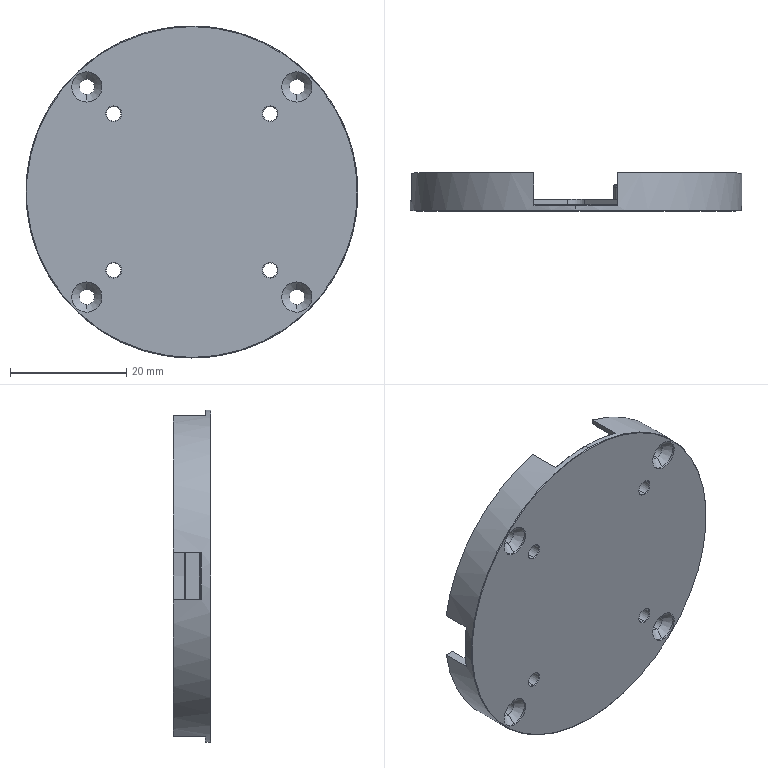Part | SolidWorks | features BaseBody 1 | 1 solid | 224 faces | box 57 x 6.5 x 57 mm | volume 5262 mm3 | cylinder 100 | plane 73 | cone 51 | commonest cylinder face diameters 4 x52 2.5 x8 2.6 x8 5.2 x8 6 x8 54 x6